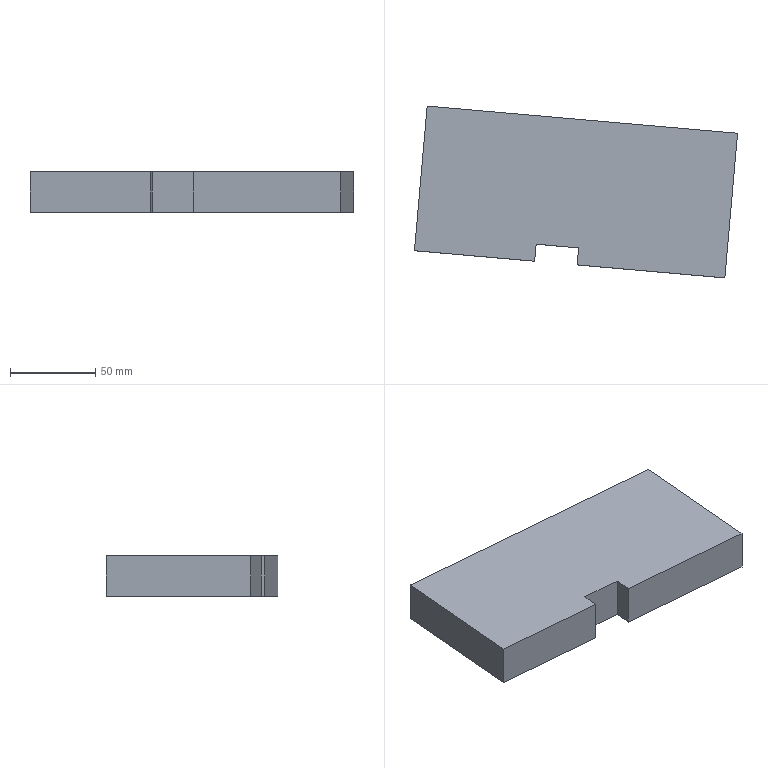Part | NX | features solid 2 | 1 solid | 10 faces | box 189.216 x 100.583 x 24 mm | volume 366302 mm3 | plane 10
STEP:
#1=CARTESIAN_POINT('',(-964.418,385.522,-246.));
#2=VERTEX_POINT('',#1);
#3=CARTESIAN_POINT('',(-964.418,385.522,-270.));
#4=VERTEX_POINT('',#3);
#5=CARTESIAN_POINT('',(-964.418,385.522,-200.289));
#6=DIRECTION('',(0.,0.,-1.));
#7=VECTOR('',#6,1000.);
#8=LINE('',#5,#7);
#9=EDGE_CURVE('',#2,#4,#8,.T.);
#10=ORIENTED_EDGE('',*,*,#9,.F.);
#11=CARTESIAN_POINT('',(-1034.801,391.679,-246.));
#12=VERTEX_POINT('',#11);
#13=CARTESIAN_POINT('',(-1034.801,391.679,-246.));
#14=DIRECTION('',(-0.9962,0.08716,0.));
#15=VECTOR('',#14,1000.);
#16=LINE('',#13,#15);
#17=EDGE_CURVE('',#12,#2,#16,.F.);
#18=ORIENTED_EDGE('',*,*,#17,.F.);
#19=CARTESIAN_POINT('',(-1034.801,391.679,-270.));
#20=VERTEX_POINT('',#19);
#21=CARTESIAN_POINT('',(-1034.801,391.679,-270.));
#22=DIRECTION('',(0.,0.,-1.));
#23=VECTOR('',#22,1000.);
#24=LINE('',#21,#23);
#25=EDGE_CURVE('',#20,#12,#24,.F.);
#26=ORIENTED_EDGE('',*,*,#25,.F.);
#27=CARTESIAN_POINT('',(-1034.801,391.679,-270.));
#28=DIRECTION('',(0.9962,-0.08716,0.));
#29=VECTOR('',#28,1000.);
#30=LINE('',#27,#29);
#31=EDGE_CURVE('',#20,#4,#30,.T.);
#32=ORIENTED_EDGE('',*,*,#31,.T.);
#33=EDGE_LOOP('',(#10,#18,#26,#32));
#34=FACE_BOUND('',#33,.T.);
#35=CARTESIAN_POINT('',(-1034.801,391.679,-270.));
#36=DIRECTION('',(-0.08716,-0.9962,0.));
#37=DIRECTION('',(0.9962,-0.08716,0.));
#38=AXIS2_PLACEMENT_3D('',#35,#36,#37);
#39=PLANE('',#38);
#40=ADVANCED_FACE('',(#34),#39,.T.);
#41=CARTESIAN_POINT('',(-939.503,383.342,-270.));
#42=VERTEX_POINT('',#41);
#43=CARTESIAN_POINT('',(-939.503,383.342,-246.));
#44=VERTEX_POINT('',#43);
#45=CARTESIAN_POINT('',(-939.503,383.342,-279.596));
#46=DIRECTION('',(0.,0.,1.));
#47=VECTOR('',#46,1000.);
#48=LINE('',#45,#47);
#49=EDGE_CURVE('',#42,#44,#48,.T.);
#50=ORIENTED_EDGE('',*,*,#49,.F.);
#51=CARTESIAN_POINT('',(-852.993,375.773,-270.));
#52=VERTEX_POINT('',#51);
#53=CARTESIAN_POINT('',(-1034.801,391.679,-270.));
#54=DIRECTION('',(0.9962,-0.08716,0.));
#55=VECTOR('',#54,1000.);
#56=LINE('',#53,#55);
#57=EDGE_CURVE('',#42,#52,#56,.T.);
#58=ORIENTED_EDGE('',*,*,#57,.T.);
#59=CARTESIAN_POINT('',(-852.993,375.773,-246.));
#60=VERTEX_POINT('',#59);
#61=CARTESIAN_POINT('',(-852.993,375.773,-270.));
#62=DIRECTION('',(0.,0.,-1.));
#63=VECTOR('',#62,1000.);
#64=LINE('',#61,#63);
#65=EDGE_CURVE('',#52,#60,#64,.F.);
#66=ORIENTED_EDGE('',*,*,#65,.T.);
#67=CARTESIAN_POINT('',(-1034.801,391.679,-246.));
#68=DIRECTION('',(-0.9962,0.08716,0.));
#69=VECTOR('',#68,1000.);
#70=LINE('',#67,#69);
#71=EDGE_CURVE('',#44,#60,#70,.F.);
#72=ORIENTED_EDGE('',*,*,#71,.F.);
#73=EDGE_LOOP('',(#50,#58,#66,#72));
#74=FACE_BOUND('',#73,.T.);
#75=CARTESIAN_POINT('',(-1034.801,391.679,-270.));
#76=DIRECTION('',(-0.08716,-0.9962,0.));
#77=DIRECTION('',(0.9962,-0.08716,0.));
#78=AXIS2_PLACEMENT_3D('',#75,#76,#77);
#79=PLANE('',#78);
#80=ADVANCED_FACE('',(#74),#79,.T.);
#81=ORIENTED_EDGE('',*,*,#17,.T.);
#82=CARTESIAN_POINT('',(-963.546,395.484,-246.));
#83=VERTEX_POINT('',#82);
#84=CARTESIAN_POINT('',(-964.418,385.522,-246.));
#85=DIRECTION('',(0.08716,0.9962,0.));
#86=VECTOR('',#85,1000.);
#87=LINE('',#84,#86);
#88=EDGE_CURVE('',#2,#83,#87,.T.);
#89=ORIENTED_EDGE('',*,*,#88,.T.);
#90=CARTESIAN_POINT('',(-938.631,393.304,-246.));
#91=VERTEX_POINT('',#90);
#92=CARTESIAN_POINT('',(-1033.929,401.641,-246.));
#93=DIRECTION('',(0.9962,-0.08716,0.));
#94=VECTOR('',#93,1000.);
#95=LINE('',#92,#94);
#96=EDGE_CURVE('',#83,#91,#95,.T.);
#97=ORIENTED_EDGE('',*,*,#96,.T.);
#98=CARTESIAN_POINT('',(-939.503,383.342,-246.));
#99=DIRECTION('',(-0.08716,-0.9962,0.));
#100=VECTOR('',#99,1000.);
#101=LINE('',#98,#100);
#102=EDGE_CURVE('',#91,#44,#101,.T.);
#103=ORIENTED_EDGE('',*,*,#102,.T.);
#104=ORIENTED_EDGE('',*,*,#71,.T.);
#105=CARTESIAN_POINT('',(-845.585,460.45,-246.));
#106=VERTEX_POINT('',#105);
#107=CARTESIAN_POINT('',(-852.993,375.773,-246.));
#108=DIRECTION('',(-0.08716,-0.9962,0.));
#109=VECTOR('',#108,1000.);
#110=LINE('',#107,#109);
#111=EDGE_CURVE('',#60,#106,#110,.F.);
#112=ORIENTED_EDGE('',*,*,#111,.T.);
#113=CARTESIAN_POINT('',(-1027.392,476.356,-246.));
#114=VERTEX_POINT('',#113);
#115=CARTESIAN_POINT('',(-1027.392,476.356,-246.));
#116=DIRECTION('',(0.9962,-0.08716,0.));
#117=VECTOR('',#116,1000.);
#118=LINE('',#115,#117);
#119=EDGE_CURVE('',#114,#106,#118,.T.);
#120=ORIENTED_EDGE('',*,*,#119,.F.);
#121=CARTESIAN_POINT('',(-1034.801,391.679,-246.));
#122=DIRECTION('',(0.08716,0.9962,0.));
#123=VECTOR('',#122,1000.);
#124=LINE('',#121,#123);
#125=EDGE_CURVE('',#12,#114,#124,.T.);
#126=ORIENTED_EDGE('',*,*,#125,.F.);
#127=EDGE_LOOP('',(#81,#89,#97,#103,#104,#112,#120,#126));
#128=FACE_BOUND('',#127,.T.);
#129=CARTESIAN_POINT('',(-1034.801,391.679,-246.));
#130=DIRECTION('',(0.,0.,1.));
#131=DIRECTION('',(0.9962,-0.08716,0.));
#132=AXIS2_PLACEMENT_3D('',#129,#130,#131);
#133=PLANE('',#132);
#134=ADVANCED_FACE('',(#128),#133,.T.);
#135=CARTESIAN_POINT('',(-963.546,395.484,-270.));
#136=VERTEX_POINT('',#135);
#137=CARTESIAN_POINT('',(-964.418,385.522,-270.));
#138=DIRECTION('',(0.08716,0.9962,0.));
#139=VECTOR('',#138,1000.);
#140=LINE('',#137,#139);
#141=EDGE_CURVE('',#4,#136,#140,.T.);
#142=ORIENTED_EDGE('',*,*,#141,.F.);
#143=ORIENTED_EDGE('',*,*,#31,.F.);
#144=CARTESIAN_POINT('',(-1027.392,476.356,-270.));
#145=VERTEX_POINT('',#144);
#146=CARTESIAN_POINT('',(-1034.801,391.679,-270.));
#147=DIRECTION('',(0.08716,0.9962,0.));
#148=VECTOR('',#147,1000.);
#149=LINE('',#146,#148);
#150=EDGE_CURVE('',#20,#145,#149,.T.);
#151=ORIENTED_EDGE('',*,*,#150,.T.);
#152=CARTESIAN_POINT('',(-845.585,460.45,-270.));
#153=VERTEX_POINT('',#152);
#154=CARTESIAN_POINT('',(-1027.392,476.356,-270.));
#155=DIRECTION('',(0.9962,-0.08716,0.));
#156=VECTOR('',#155,1000.);
#157=LINE('',#154,#156);
#158=EDGE_CURVE('',#145,#153,#157,.T.);
#159=ORIENTED_EDGE('',*,*,#158,.T.);
#160=CARTESIAN_POINT('',(-852.993,375.773,-270.));
#161=DIRECTION('',(0.08716,0.9962,0.));
#162=VECTOR('',#161,1000.);
#163=LINE('',#160,#162);
#164=EDGE_CURVE('',#52,#153,#163,.T.);
#165=ORIENTED_EDGE('',*,*,#164,.F.);
#166=ORIENTED_EDGE('',*,*,#57,.F.);
#167=CARTESIAN_POINT('',(-938.631,393.304,-270.));
#168=VERTEX_POINT('',#167);
#169=CARTESIAN_POINT('',(-939.503,383.342,-270.));
#170=DIRECTION('',(-0.08716,-0.9962,0.));
#171=VECTOR('',#170,1000.);
#172=LINE('',#169,#171);
#173=EDGE_CURVE('',#168,#42,#172,.T.);
#174=ORIENTED_EDGE('',*,*,#173,.F.);
#175=CARTESIAN_POINT('',(-1033.929,401.641,-270.));
#176=DIRECTION('',(0.9962,-0.08716,0.));
#177=VECTOR('',#176,1000.);
#178=LINE('',#175,#177);
#179=EDGE_CURVE('',#136,#168,#178,.T.);
#180=ORIENTED_EDGE('',*,*,#179,.F.);
#181=EDGE_LOOP('',(#142,#143,#151,#159,#165,#166,#174,#180));
#182=FACE_BOUND('',#181,.T.);
#183=CARTESIAN_POINT('',(-1034.801,391.679,-270.));
#184=DIRECTION('',(0.,0.,1.));
#185=DIRECTION('',(0.9962,-0.08716,0.));
#186=AXIS2_PLACEMENT_3D('',#183,#184,#185);
#187=PLANE('',#186);
#188=ADVANCED_FACE('',(#182),#187,.F.);
#189=ORIENTED_EDGE('',*,*,#25,.T.);
#190=ORIENTED_EDGE('',*,*,#125,.T.);
#191=CARTESIAN_POINT('',(-1027.392,476.356,-270.));
#192=DIRECTION('',(0.,0.,-1.));
#193=VECTOR('',#192,1000.);
#194=LINE('',#191,#193);
#195=EDGE_CURVE('',#145,#114,#194,.F.);
#196=ORIENTED_EDGE('',*,*,#195,.F.);
#197=ORIENTED_EDGE('',*,*,#150,.F.);
#198=EDGE_LOOP('',(#189,#190,#196,#197));
#199=FACE_BOUND('',#198,.T.);
#200=CARTESIAN_POINT('',(-1034.801,391.679,-270.));
#201=DIRECTION('',(0.9962,-0.08716,0.));
#202=DIRECTION('',(0.08716,0.9962,0.));
#203=AXIS2_PLACEMENT_3D('',#200,#201,#202);
#204=PLANE('',#203);
#205=ADVANCED_FACE('',(#199),#204,.F.);
#206=ORIENTED_EDGE('',*,*,#195,.T.);
#207=ORIENTED_EDGE('',*,*,#119,.T.);
#208=CARTESIAN_POINT('',(-845.585,460.45,-270.));
#209=DIRECTION('',(0.,0.,-1.));
#210=VECTOR('',#209,1000.);
#211=LINE('',#208,#210);
#212=EDGE_CURVE('',#153,#106,#211,.F.);
#213=ORIENTED_EDGE('',*,*,#212,.F.);
#214=ORIENTED_EDGE('',*,*,#158,.F.);
#215=EDGE_LOOP('',(#206,#207,#213,#214));
#216=FACE_BOUND('',#215,.T.);
#217=CARTESIAN_POINT('',(-1027.392,476.356,-270.));
#218=DIRECTION('',(-0.08716,-0.9962,0.));
#219=DIRECTION('',(0.9962,-0.08716,0.));
#220=AXIS2_PLACEMENT_3D('',#217,#218,#219);
#221=PLANE('',#220);
#222=ADVANCED_FACE('',(#216),#221,.F.);
#223=ORIENTED_EDGE('',*,*,#164,.T.);
#224=ORIENTED_EDGE('',*,*,#212,.T.);
#225=ORIENTED_EDGE('',*,*,#111,.F.);
#226=ORIENTED_EDGE('',*,*,#65,.F.);
#227=EDGE_LOOP('',(#223,#224,#225,#226));
#228=FACE_BOUND('',#227,.T.);
#229=CARTESIAN_POINT('',(-852.993,375.773,-270.));
#230=DIRECTION('',(0.9962,-0.08716,0.));
#231=DIRECTION('',(0.08716,0.9962,0.));
#232=AXIS2_PLACEMENT_3D('',#229,#230,#231);
#233=PLANE('',#232);
#234=ADVANCED_FACE('',(#228),#233,.T.);
#235=ORIENTED_EDGE('',*,*,#9,.T.);
#236=ORIENTED_EDGE('',*,*,#141,.T.);
#237=CARTESIAN_POINT('',(-963.546,395.484,-200.289));
#238=DIRECTION('',(0.,0.,-1.));
#239=VECTOR('',#238,1000.);
#240=LINE('',#237,#239);
#241=EDGE_CURVE('',#83,#136,#240,.T.);
#242=ORIENTED_EDGE('',*,*,#241,.F.);
#243=ORIENTED_EDGE('',*,*,#88,.F.);
#244=EDGE_LOOP('',(#235,#236,#242,#243));
#245=FACE_BOUND('',#244,.T.);
#246=CARTESIAN_POINT('',(-964.418,385.522,-200.289));
#247=DIRECTION('',(0.9962,-0.08716,0.));
#248=DIRECTION('',(0.,0.,-1.));
#249=AXIS2_PLACEMENT_3D('',#246,#247,#248);
#250=PLANE('',#249);
#251=ADVANCED_FACE('',(#245),#250,.T.);
#252=CARTESIAN_POINT('',(-938.631,393.304,-279.596));
#253=DIRECTION('',(0.,0.,1.));
#254=VECTOR('',#253,1000.);
#255=LINE('',#252,#254);
#256=EDGE_CURVE('',#168,#91,#255,.T.);
#257=ORIENTED_EDGE('',*,*,#256,.F.);
#258=ORIENTED_EDGE('',*,*,#173,.T.);
#259=ORIENTED_EDGE('',*,*,#49,.T.);
#260=ORIENTED_EDGE('',*,*,#102,.F.);
#261=EDGE_LOOP('',(#257,#258,#259,#260));
#262=FACE_BOUND('',#261,.T.);
#263=CARTESIAN_POINT('',(-939.503,383.342,-279.596));
#264=DIRECTION('',(-0.9962,0.08716,0.));
#265=DIRECTION('',(0.,0.,1.));
#266=AXIS2_PLACEMENT_3D('',#263,#264,#265);
#267=PLANE('',#266);
#268=ADVANCED_FACE('',(#262),#267,.T.);
#269=ORIENTED_EDGE('',*,*,#241,.T.);
#270=ORIENTED_EDGE('',*,*,#179,.T.);
#271=ORIENTED_EDGE('',*,*,#256,.T.);
#272=ORIENTED_EDGE('',*,*,#96,.F.);
#273=EDGE_LOOP('',(#269,#270,#271,#272));
#274=FACE_BOUND('',#273,.T.);
#275=CARTESIAN_POINT('',(-963.546,395.484,-279.596));
#276=DIRECTION('',(-0.08716,-0.9962,0.));
#277=DIRECTION('',(0.,0.,-1.));
#278=AXIS2_PLACEMENT_3D('',#275,#276,#277);
#279=PLANE('',#278);
#280=ADVANCED_FACE('',(#274),#279,.T.);
#281=CLOSED_SHELL('',(#40,#80,#134,#188,#205,#222,#234,#251,#268,#280));
#282=MANIFOLD_SOLID_BREP('',#281);
#283=(LENGTH_UNIT()NAMED_UNIT(*)SI_UNIT(.MILLI.,.METRE.));
#284=UNCERTAINTY_MEASURE_WITH_UNIT(LENGTH_MEASURE(0.00001),#283,'','');
#285=(NAMED_UNIT(*)PLANE_ANGLE_UNIT()SI_UNIT($,.RADIAN.));
#286=(NAMED_UNIT(*)SI_UNIT($,.STERADIAN.)SOLID_ANGLE_UNIT());
#287=(GEOMETRIC_REPRESENTATION_CONTEXT(3)GLOBAL_UNCERTAINTY_ASSIGNED_CONTEXT((#284))GLOBAL_UNIT_ASSIGNED_CONTEXT((#283,#285,#286))REPRESENTATION_CONTEXT('',''));
#288=ADVANCED_BREP_SHAPE_REPRESENTATION('',(#282),#287);